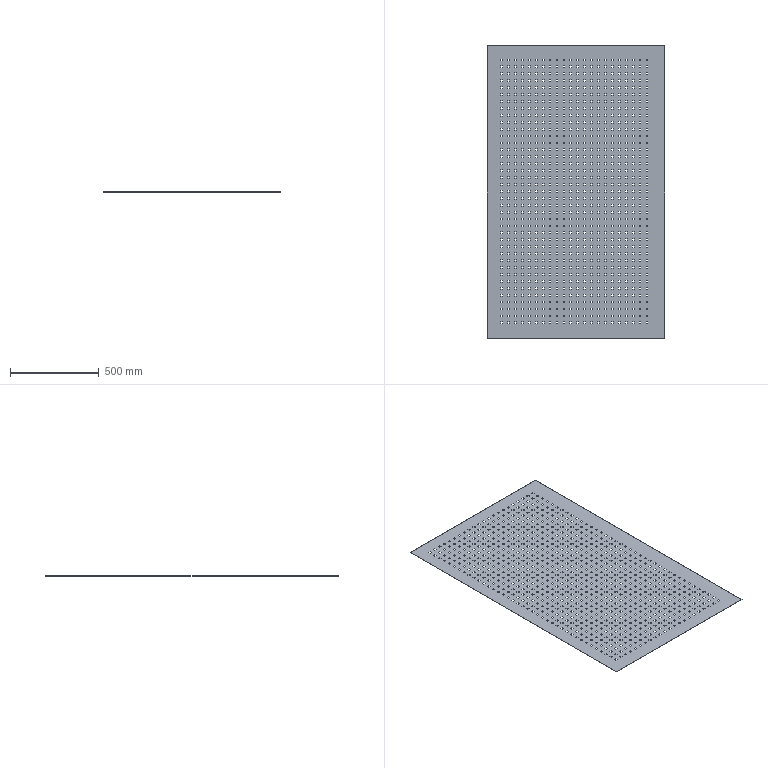Part | SolidWorks | features Extrusion 1, ICE 1, LPattern 1 | 1 solid | 3438 faces | volume 1559902 mm3 | plane 3438